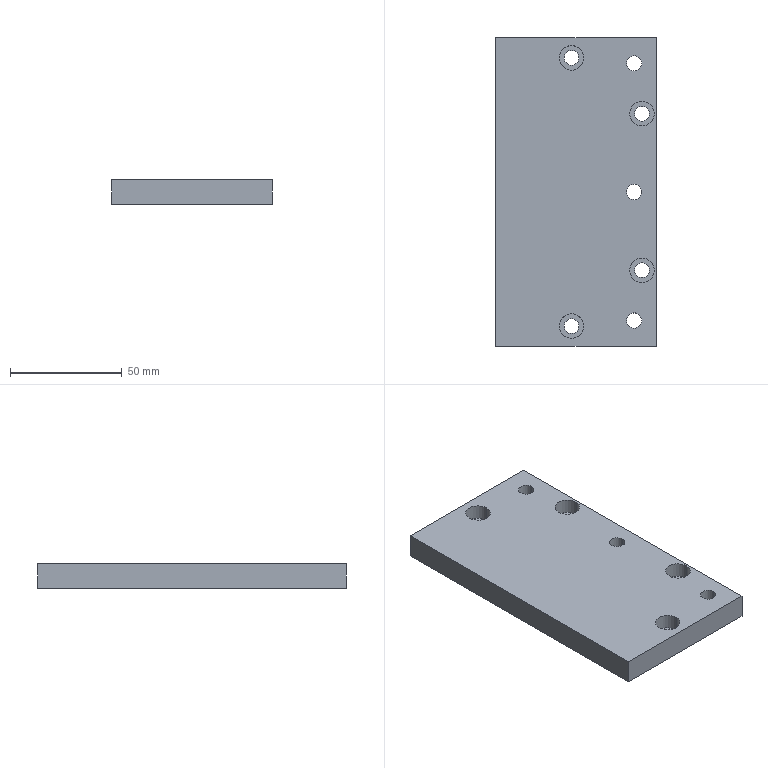Part | STEP file | PN_0021 cover block | 1 solid | 32 faces | box 72 x 138 x 11 mm | volume 104938 mm3 | cylinder 22 | plane 10 | commonest cylinder face diameters 6.6 x8 11 x8 6.8 x6